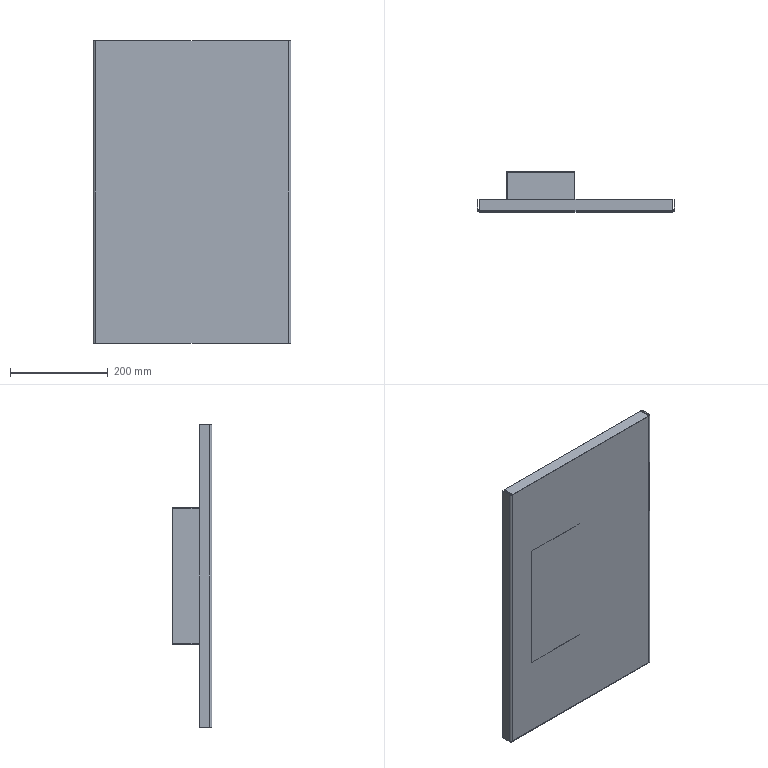Part | STEP file | ASND-0110-E63-HLTP01标准Lower机架-06(Default) | 1 solid | 39 faces | box 405 x 81.5 x 620 mm | volume 552144 mm3 | plane 33 | cylinder 6 | commonest cylinder face diameters 7 x2 10 x2 40 x2